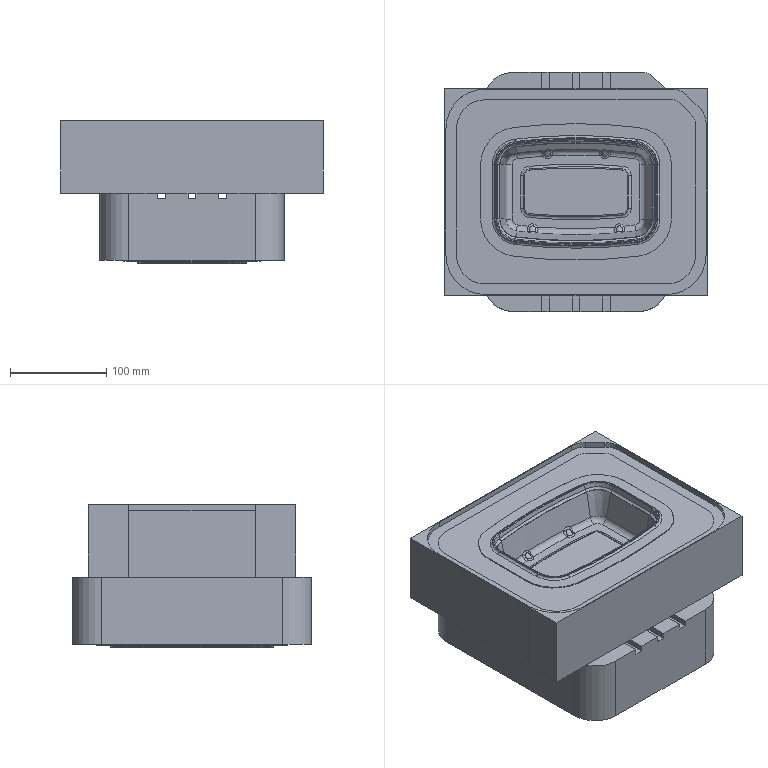NC program | NX | posted with a generic post | part box 272.387 x 248.388 x 148.5 mm
Lines 1 to 1186 of 133013:
N10 G17 G21 G94 G90
(CAVITY_MILL_1 , TOOL : D16R0.8)
N12 T00 M6
N14 G53
N16 G17 G0 G90 X-26.555 Y98.736 S7000 M3 M8
N18 G43 Z133. H0
N20 Z76.5
N22 G94 G1 X0. Z75.108 F4500.
N24 X100.052
N26 G2 X109.203 Y94.945 R12.942
N28 G1 X123.345 Y80.803
N30 G2 X127.136 Y71.651 R12.942
N32 G1 Y-65.794
N34 G2 X94.194 Y-98.736 R32.942
N36 G1 X-94.194
N38 G2 X-127.136 Y-65.794 R32.942
N40 G1 Y65.794
N42 G2 X-94.194 Y98.736 R32.942
N44 G1 X0.
N46 Y88.656
N48 X100.052
N50 G2 X102.076 Y87.817 R2.862
N52 G1 X116.218 Y73.675
N54 G2 X117.056 Y71.651 R2.862
N56 G1 Y-65.794
N58 G2 X94.194 Y-88.656 R22.862
N60 G1 X-94.194
N62 G2 X-117.056 Y-65.794 R22.862
N64 G1 Y65.794
N66 G2 X-94.194 Y88.656 R22.862
N68 G1 X0.
N70 Y78.576
N72 X97.062
N74 X106.976 Y68.662
N76 Y-65.794
N78 G2 X94.194 Y-78.576 R12.782
N80 G1 X-94.194
N82 G2 X-106.976 Y-65.794 R12.782
N84 G1 Y65.794
N86 G2 X-94.194 Y78.576 R12.782
N88 G1 X0.
N90 Y68.496
N92 X92.887
N94 X96.896 Y64.486
N96 Y-65.794
N98 G2 X94.194 Y-68.496 R2.702
N100 G1 X-94.194
N102 G2 X-96.896 Y-65.794 R2.702
N104 G1 Y65.794
N106 G2 X-94.194 Y68.496 R2.702
N108 G1 X0.
N110 Y58.416
N112 X86.816
N114 Y-58.416
N116 X-86.816
N118 Y58.416
N120 X0.
N122 Y48.336
N124 X76.736
N126 Y-48.336
N128 X-76.736
N130 Y48.336
N132 X0.
N134 Y38.256
N136 X66.656
N138 Y-38.256
N140 X-66.656
N142 Y38.256
N144 X0.
N146 Y28.176
N148 X56.576
N150 Y-28.176
N152 X-56.576
N154 Y28.176
N156 X0.
N158 Y18.096
N160 X46.496
N162 Y-18.096
N164 X-46.496
N166 Y18.096
N168 X0.
N170 Y8.016
N172 X36.416
N174 Y-8.016
N176 X-36.416
N178 Y8.016
N180 X0.
N182 Y0.816
N184 X29.216
N186 Y-0.816
N188 X-29.216
N190 Y0.816
N192 X0.
N194 G3 X3.2 Y4.016 R3.2
N196 G1 Z76.108
N198 G0 Z78.5
N200 X-26.555 Y98.644
N202 Z76.108
N204 G1 X0. Z74.717
N206 X100.052
N208 G2 X109.138 Y94.88 R12.85
N210 G1 X123.251 Y80.767
N212 X123.296 Y80.722
N214 G2 X127.044 Y71.651 R12.85
N216 G1 Y-65.794
N218 G2 X94.194 Y-98.644 R32.85
N220 G1 X-94.194
N222 G2 X-127.044 Y-65.794 R32.85
N224 G1 Y65.794
N226 G2 X-94.194 Y98.644 R32.85
N228 G1 X0.
N230 Y88.564
N232 X100.052
N234 G2 X102.01 Y87.752 R2.77
N236 G1 X116.123 Y73.64
N238 G2 X116.964 Y71.651 R2.77
N240 G1 Y-65.794
N242 G2 X94.194 Y-88.564 R22.77
N244 G1 X-94.194
N246 G2 X-116.964 Y-65.794 R22.77
N248 G1 Y65.794
N250 G2 X-94.194 Y88.564 R22.77
N252 G1 X0.
N254 Y78.484
N256 X97.024
N258 X106.884 Y68.624
N260 Y-65.794
N262 G2 X94.194 Y-78.484 R12.69
N264 G1 X-94.194
N266 G2 X-106.884 Y-65.794 R12.69
N268 G1 Y65.794
N270 G2 X-94.194 Y78.484 R12.69
N272 G1 X0.
N274 Y68.404
N276 X92.849
N278 X96.804 Y64.448
N280 Y-65.794
N282 G2 X94.194 Y-68.404 R2.61
N284 G1 X-94.194
N286 G2 X-96.804 Y-65.794 R2.61
N288 G1 Y65.794
N290 G2 X-94.194 Y68.404 R2.61
N292 G1 X0.
N294 Y58.324
N296 X86.724
N298 Y-58.324
N300 X-86.724
N302 Y58.324
N304 X0.
N306 Y48.244
N308 X76.644
N310 Y-48.244
N312 X-76.644
N314 Y48.244
N316 X0.
N318 Y38.164
N320 X66.564
N322 Y-38.164
N324 X-66.564
N326 Y38.164
N328 X0.
N330 Y28.084
N332 X56.484
N334 Y-28.084
N336 X-56.484
N338 Y28.084
N340 X0.
N342 Y18.004
N344 X46.404
N346 Y-18.004
N348 X-46.404
N350 Y18.004
N352 X0.
N354 Y7.924
N356 X36.324
N358 Y-7.924
N360 X-36.324
N362 Y7.924
N364 X0.
N366 Y0.724
N368 X29.124
N370 Y-0.724
N372 X-29.124
N374 Y0.724
N376 X0.
N378 G3 X3.2 Y3.924 R3.2
N380 G1 Z75.717
N382 G0 Z78.108
N384 X-26.555 Y98.644
N386 Z75.717
N388 G1 X0. Z74.325
N390 X100.052
N392 G2 X109.138 Y94.88 R12.85
N394 G1 X123.28 Y80.738
N396 G2 X127.044 Y71.651 R12.85
N398 G1 Y-65.794
N400 G2 X94.194 Y-98.644 R32.85
N402 G1 X-94.194
N404 G2 X-127.044 Y-65.794 R32.85
N406 G1 Y65.794
N408 G2 X-94.194 Y98.644 R32.85
N410 G1 X0.
N412 Y88.564
N414 X100.052
N416 G2 X102.01 Y87.752 R2.77
N418 G1 X116.152 Y73.61
N420 G2 X116.964 Y71.651 R2.77
N422 G1 Y-65.794
N424 G2 X94.194 Y-88.564 R22.77
N426 G1 X-94.194
N428 G2 X-116.964 Y-65.794 R22.77
N430 G1 Y65.794
N432 G2 X-94.194 Y88.564 R22.77
N434 G1 X0.
N436 Y78.484
N438 X97.024
N440 X106.884 Y68.623
N442 Y-65.794
N444 G2 X94.194 Y-78.484 R12.69
N446 G1 X-94.194
N448 G2 X-106.884 Y-65.794 R12.69
N450 G1 Y65.794
N452 G2 X-94.194 Y78.484 R12.69
N454 G1 X0.
N456 Y68.404
N458 X92.848
N460 X96.804 Y64.448
N462 Y-65.794
N464 G2 X94.194 Y-68.404 R2.61
N466 G1 X-94.194
N468 G2 X-96.804 Y-65.794 R2.61
N470 G1 Y65.794
N472 G2 X-94.194 Y68.404 R2.61
N474 G1 X0.
N476 Y58.324
N478 X86.724
N480 Y-58.324
N482 X-86.724
N484 Y58.324
N486 X0.
N488 Y48.244
N490 X76.644
N492 Y-48.244
N494 X-76.644
N496 Y48.244
N498 X0.
N500 Y38.164
N502 X66.564
N504 Y-38.164
N506 X-66.564
N508 Y38.164
N510 X0.
N512 Y28.084
N514 X56.484
N516 Y-28.084
N518 X-56.484
N520 Y28.084
N522 X0.
N524 Y18.004
N526 X46.404
N528 Y-18.004
N530 X-46.404
N532 Y18.004
N534 X0.
N536 Y7.924
N538 X36.324
N540 Y-7.924
N542 X-36.324
N544 Y7.924
N546 X0.
N548 Y0.724
N550 X29.124
N552 Y-0.724
N554 X-29.124
N556 Y0.724
N558 X0.
N560 G3 X3.2 Y3.924 R3.2
N562 G1 Z75.325
N564 G0 Z77.717
N566 X-26.555 Y98.644
N568 Z75.325
N570 G1 X0. Z73.933
N572 X100.052
N574 G2 X109.138 Y94.88 R12.85
N576 G1 X123.28 Y80.738
N578 G2 X127.044 Y71.651 R12.85
N580 G1 Y-65.794
N582 G2 X94.194 Y-98.644 R32.85
N584 G1 X-94.194
N586 G2 X-127.044 Y-65.794 R32.85
N588 G1 Y65.794
N590 G2 X-94.194 Y98.644 R32.85
N592 G1 X0.
N594 Y88.564
N596 X100.052
N598 G2 X102.01 Y87.752 R2.77
N600 G1 X116.152 Y73.61
N602 G2 X116.964 Y71.651 R2.77
N604 G1 Y-65.794
N606 G2 X94.194 Y-88.564 R22.77
N608 G1 X-94.194
N610 G2 X-116.964 Y-65.794 R22.77
N612 G1 Y65.794
N614 G2 X-94.194 Y88.564 R22.77
N616 G1 X0.
N618 Y78.484
N620 X97.024
N622 X106.884 Y68.623
N624 Y-65.794
N626 G2 X94.194 Y-78.484 R12.69
N628 G1 X-94.194
N630 G2 X-106.884 Y-65.794 R12.69
N632 G1 Y65.794
N634 G2 X-94.194 Y78.484 R12.69
N636 G1 X0.
N638 Y68.404
N640 X92.848
N642 X96.804 Y64.448
N644 Y-65.794
N646 G2 X94.194 Y-68.404 R2.61
N648 G1 X-94.194
N650 G2 X-96.804 Y-65.794 R2.61
N652 G1 Y65.794
N654 G2 X-94.194 Y68.404 R2.61
N656 G1 X0.
N658 Y58.324
N660 X86.724
N662 Y-58.324
N664 X-86.724
N666 Y58.324
N668 X0.
N670 Y48.244
N672 X76.644
N674 Y-48.244
N676 X-76.644
N678 Y48.244
N680 X0.
N682 Y38.164
N684 X66.564
N686 Y-38.164
N688 X-66.564
N690 Y38.164
N692 X0.
N694 Y28.084
N696 X56.484
N698 Y-28.084
N700 X-56.484
N702 Y28.084
N704 X0.
N706 Y18.004
N708 X46.404
N710 Y-18.004
N712 X-46.404
N714 Y18.004
N716 X0.
N718 Y7.924
N720 X36.324
N722 Y-7.924
N724 X-36.324
N726 Y7.924
N728 X0.
N730 Y0.724
N732 X29.124
N734 Y-0.724
N736 X-29.124
N738 Y0.724
N740 X0.
N742 G3 X3.2 Y3.924 R3.2
N744 G1 Z74.933
N746 G0 Z77.325
N748 X-26.555 Y98.644
N750 Z74.933
N752 G1 X0. Z73.542
N754 X100.052
N756 G2 X109.138 Y94.88 R12.85
N758 G1 X123.28 Y80.738
N760 G2 X127.044 Y71.651 R12.85
N762 G1 Y-65.794
N764 G2 X94.194 Y-98.644 R32.85
N766 G1 X-94.194
N768 G2 X-127.044 Y-65.794 R32.85
N770 G1 Y65.794
N772 G2 X-94.194 Y98.644 R32.85
N774 G1 X0.
N776 Y88.564
N778 X100.052
N780 G2 X102.01 Y87.752 R2.77
N782 G1 X116.152 Y73.61
N784 G2 X116.964 Y71.651 R2.77
N786 G1 Y-65.794
N788 G2 X94.194 Y-88.564 R22.77
N790 G1 X-94.194
N792 G2 X-116.964 Y-65.794 R22.77
N794 G1 Y65.794
N796 G2 X-94.194 Y88.564 R22.77
N798 G1 X0.
N800 Y78.484
N802 X97.024
N804 X106.884 Y68.623
N806 Y-65.794
N808 G2 X94.194 Y-78.484 R12.69
N810 G1 X-94.194
N812 G2 X-106.884 Y-65.794 R12.69
N814 G1 Y65.794
N816 G2 X-94.194 Y78.484 R12.69
N818 G1 X0.
N820 Y68.404
N822 X92.848
N824 X96.804 Y64.448
N826 Y-65.794
N828 G2 X94.194 Y-68.404 R2.61
N830 G1 X-94.194
N832 G2 X-96.804 Y-65.794 R2.61
N834 G1 Y65.794
N836 G2 X-94.194 Y68.404 R2.61
N838 G1 X0.
N840 Y58.324
N842 X86.724
N844 Y-58.324
N846 X-86.724
N848 Y58.324
N850 X0.
N852 Y48.244
N854 X76.644
N856 Y-48.244
N858 X-76.644
N860 Y48.244
N862 X0.
N864 Y38.164
N866 X66.564
N868 Y-38.164
N870 X-66.564
N872 Y38.164
N874 X0.
N876 Y28.084
N878 X56.484
N880 Y-28.084
N882 X-56.484
N884 Y28.084
N886 X0.
N888 Y18.004
N890 X46.404
N892 Y-18.004
N894 X-46.404
N896 Y18.004
N898 X0.
N900 Y7.924
N902 X36.324
N904 Y-7.924
N906 X-36.324
N908 Y7.924
N910 X0.
N912 Y0.724
N914 X29.124
N916 Y-0.724
N918 X-29.124
N920 Y0.724
N922 X0.
N924 G3 X3.2 Y3.924 R3.2
N926 G1 Z74.542
N928 G0 Z76.933
N930 X-26.555 Y98.644
N932 Z74.542
N934 G1 X0. Z73.15
N936 X100.052
N938 G2 X109.138 Y94.88 R12.85
N940 G1 X123.28 Y80.738
N942 G2 X127.044 Y71.651 R12.85
N944 G1 Y-65.794
N946 G2 X94.194 Y-98.644 R32.85
N948 G1 X-94.194
N950 G2 X-127.044 Y-65.794 R32.85
N952 G1 Y65.794
N954 G2 X-94.194 Y98.644 R32.85
N956 G1 X0.
N958 Y88.564
N960 X100.052
N962 G2 X102.01 Y87.752 R2.77
N964 G1 X116.152 Y73.61
N966 G2 X116.964 Y71.651 R2.77
N968 G1 Y-65.794
N970 G2 X94.194 Y-88.564 R22.77
N972 G1 X-94.194
N974 G2 X-116.964 Y-65.794 R22.77
N976 G1 Y65.794
N978 G2 X-94.194 Y88.564 R22.77
N980 G1 X0.
N982 Y78.484
N984 X97.024
N986 X106.884 Y68.623
N988 Y-65.794
N990 G2 X94.194 Y-78.484 R12.69
N992 G1 X-94.194
N994 G2 X-106.884 Y-65.794 R12.69
N996 G1 Y65.794
N998 G2 X-94.194 Y78.484 R12.69
N1000 G1 X0.
N1002 Y68.404
N1004 X92.848
N1006 X96.804 Y64.448
N1008 Y-65.794
N1010 G2 X94.194 Y-68.404 R2.61
N1012 G1 X-94.194
N1014 G2 X-96.804 Y-65.794 R2.61
N1016 G1 Y65.794
N1018 G2 X-94.194 Y68.404 R2.61
N1020 G1 X0.
N1022 Y58.324
N1024 X86.724
N1026 Y-58.324
N1028 X-86.724
N1030 Y58.324
N1032 X0.
N1034 Y48.244
N1036 X76.644
N1038 Y-48.244
N1040 X-76.644
N1042 Y48.244
N1044 X0.
N1046 Y38.164
N1048 X66.564
N1050 Y-38.164
N1052 X-66.564
N1054 Y38.164
N1056 X0.
N1058 Y28.084
N1060 X56.484
N1062 Y-28.084
N1064 X-56.484
N1066 Y28.084
N1068 X0.
N1070 Y18.004
N1072 X46.404
N1074 Y-18.004
N1076 X-46.404
N1078 Y18.004
N1080 X0.
N1082 Y7.924
N1084 X36.324
N1086 Y-7.924
N1088 X-36.324
N1090 Y7.924
N1092 X0.
N1094 Y0.724
N1096 X29.124
N1098 Y-0.724
N1100 X-29.124
N1102 Y0.724
N1104 X0.
N1106 G3 X3.2 Y3.924 R3.2
N1108 G1 Z74.15
N1110 G0 Z76.542
N1112 X-26.373 Y98.644
N1114 Z74.15
N1116 G1 X0. Z72.768
N1118 X100.052
N1120 G2 X109.138 Y94.88 R12.85
N1122 G1 X123.28 Y80.738
N1124 G2 X127.044 Y71.651 R12.85
N1126 G1 Y-65.794
N1128 G2 X94.194 Y-98.644 R32.85
N1130 G1 X-94.194
N1132 G2 X-127.044 Y-65.794 R32.85
N1134 G1 Y65.794
N1136 G2 X-94.194 Y98.644 R32.85
N1138 G1 X0.
N1140 Y88.564
N1142 X100.052
N1144 G2 X102.01 Y87.752 R2.77
N1146 G1 X116.152 Y73.61
N1148 G2 X116.964 Y71.651 R2.77
N1150 G1 Y-65.794
N1152 G2 X94.194 Y-88.564 R22.77
N1154 G1 X-94.194
N1156 G2 X-116.964 Y-65.794 R22.77
N1158 G1 Y65.794
N1160 G2 X-94.194 Y88.564 R22.77
N1162 G1 X0.
N1164 Y78.484
N1166 X97.024
N1168 X106.884 Y68.623
N1170 Y-65.794
N1172 G2 X94.194 Y-78.484 R12.69
N1174 G1 X-94.194
N1176 G2 X-106.884 Y-65.794 R12.69
N1178 G1 Y65.794
N1180 G2 X-94.194 Y78.484 R12.69
N1182 G1 X0.
N1184 Y68.404
N1186 X92.848
N1188 X96.804 Y64.448
N1190 Y49.668
N1192 X86.724
N1194 G3 X76.172 Y58.324 R34.054
N1196 G1 X69.25 Y61.133
N1198 X76.172 Y58.324
N1200 X86.724
N1202 Y49.668
N1204 X96.804
N1206 Y-65.794
N1208 G2 X94.194 Y-68.404 R2.61
N1210 G1 X76.392
N1212 Y-58.324
N1214 G3 X86.724 Y-49.919 R33.509
N1216 G1 Y-58.324
N1218 X76.392
N1220 X69.418 Y-61.124
N1222 X76.392 Y-58.324
N1224 Y-68.404
N1226 X-94.194
N1228 G2 X-96.804 Y-65.794 R2.61
N1230 G1 Y-49.668
N1232 X-86.724
N1234 G3 X-76.172 Y-58.324 R34.054
N1236 G1 X-69.25 Y-61.133
N1238 X-76.172 Y-58.324
N1240 X-86.724
N1242 Y-49.668
N1244 X-96.804
N1246 Y65.794
N1248 G2 X-94.194 Y68.404 R2.61
N1250 G1 X-76.172
N1252 Y58.324
N1254 G3 X-86.724 Y49.668 R34.054
N1256 G1 X-85.159 Y48.397
N1258 G2 X-64.169 Y60.003 R32.038
N1260 X64.169 Y60.003 R526.731
N1262 X92.327 Y28.201 R32.038
N1264 G1 Y-28.645
N1266 G2 X66.064 Y-59.701 R31.493
N1268 G1 X64.545 Y-59.957
N1270 G2 X-64.193 Y-60. R526.731
N1272 X-92.327 Y-28.201 R32.038
N1274 G1 Y28.201
N1276 G2 X-85.159 Y48.397 R32.038
N1278 G1 X-86.724 Y49.668
N1280 Y58.324
N1282 X-76.172
N1284 X-69.25 Y61.133
N1286 X-76.172 Y58.324
N1288 Y68.404
N1290 X0.
N1292 G3 X3.2 Y71.604 R3.2
N1294 G1 Z73.768
N1296 G0 Z76.15
N1298 X-26.373 Y98.644
N1300 Z73.768
N1302 G1 X0. Z72.386
N1304 X100.052
N1306 G2 X109.138 Y94.88 R12.85
N1308 G1 X123.28 Y80.738
N1310 G2 X127.044 Y71.651 R12.85
N1312 G1 Y-65.794
N1314 G2 X94.194 Y-98.644 R32.85
N1316 G1 X-94.194
N1318 G2 X-127.044 Y-65.794 R32.85
N1320 G1 Y65.794
N1322 G2 X-94.194 Y98.644 R32.85
N1324 G1 X0.
N1326 Y88.564
N1328 X100.052
N1330 G2 X102.01 Y87.752 R2.77
N1332 G1 X116.152 Y73.61
N1334 G2 X116.964 Y71.651 R2.77
N1336 G1 Y-65.794
N1338 G2 X94.194 Y-88.564 R22.77
N1340 G1 X-94.194
N1342 G2 X-116.964 Y-65.794 R22.77
N1344 G1 Y65.794
N1346 G2 X-94.194 Y88.564 R22.77
N1348 G1 X0.
N1350 Y78.484
N1352 X97.024
N1354 X106.884 Y68.623
N1356 Y-65.794
N1358 G2 X94.194 Y-78.484 R12.69
N1360 G1 X-94.194
N1362 G2 X-106.884 Y-65.794 R12.69
N1364 G1 Y65.794
N1366 G2 X-94.194 Y78.484 R12.69
N1368 G1 X0.
N1370 Y68.404
N1372 X92.848
N1374 X96.804 Y64.448
N1376 Y50.136
N1378 X86.724
N1380 G3 X76.799 Y58.324 R34.351
N1382 G1 X70.058 Y61.17
N1384 X76.799 Y58.324
N1386 X86.724
N1388 Y50.136
N1390 X96.804
N1392 Y-65.794
N1394 G2 X94.194 Y-68.404 R2.61
N1396 G1 X77.038
N1398 Y-58.324
N1400 G3 X86.724 Y-50.398 R33.78
N1402 G1 Y-58.324
N1404 X77.038
N1406 X70.259 Y-61.162
N1408 X77.038 Y-58.324
N1410 Y-68.404
N1412 X-94.194
N1414 G2 X-96.804 Y-65.794 R2.61
N1416 G1 Y-50.136
N1418 X-86.724
N1420 G3 X-76.799 Y-58.324 R34.351
N1422 G1 X-70.058 Y-61.17
N1424 X-76.799 Y-58.324
N1426 X-86.724
N1428 Y-50.136
N1430 X-96.804
N1432 Y65.794
N1434 G2 X-94.194 Y68.404 R2.61
N1436 G1 X-76.799
N1438 Y58.324
N1440 G3 X-86.724 Y50.136 R34.351
N1442 G1 X-85.172 Y48.849
N1444 G2 X-64.229 Y60.295 R32.335
N1446 X64.229 Y60.295 R527.028
N1448 X92.623 Y28.201 R32.335
N1450 G1 Y-28.519
N1452 G2 X86.607 Y-47.271 R32.261
N1454 X68.014 Y-59.618 R31.764
N1456 X64.582 Y-60.251 R32.117
N1458 X-64.229 Y-60.295 R527.028
N1460 X-92.623 Y-28.201 R32.335
N1462 G1 Y28.201
N1464 G2 X-85.172 Y48.849 R32.335
N1466 G1 X-86.724 Y50.136
N1468 Y58.324
N1470 X-76.799
N1472 X-70.058 Y61.17
N1474 X-76.799 Y58.324
N1476 Y68.404
N1478 X0.
N1480 G3 X3.2 Y71.604 R3.2
N1482 G1 Z73.386
N1484 G0 Z75.768
N1486 X-26.373 Y98.644
N1488 Z73.386
N1490 G1 X0. Z72.004
N1492 X100.052
N1494 G2 X109.138 Y94.88 R12.85
N1496 G1 X123.28 Y80.738
N1498 G2 X127.044 Y71.651 R12.85
N1500 G1 Y-65.794
N1502 G2 X94.194 Y-98.644 R32.85
N1504 G1 X-94.194
N1506 G2 X-127.044 Y-65.794 R32.85
N1508 G1 Y65.794
N1510 G2 X-94.194 Y98.644 R32.85
N1512 G1 X0.
N1514 Y88.564
N1516 X100.052
N1518 G2 X102.01 Y87.752 R2.77
N1520 G1 X116.152 Y73.61
N1522 G2 X116.964 Y71.651 R2.77
N1524 G1 Y-65.794
N1526 G2 X94.194 Y-88.564 R22.77
N1528 G1 X-94.194
N1530 G2 X-116.964 Y-65.794 R22.77
N1532 G1 Y65.794
N1534 G2 X-94.194 Y88.564 R22.77
N1536 G1 X0.
N1538 Y78.484
N1540 X97.024
N1542 X106.884 Y68.623
N1544 Y-65.794
N1546 G2 X94.194 Y-78.484 R12.69
N1548 G1 X-94.194
N1550 G2 X-106.884 Y-65.794 R12.69
N1552 G1 Y65.794
N1554 G2 X-94.194 Y78.484 R12.69
N1556 G1 X0.
N1558 Y68.404
N1560 X92.848
N1562 X96.804 Y64.448
N1564 Y50.355
N1566 X86.724
N1568 G3 X77.089 Y58.324 R34.491
N1570 G1 X70.423 Y61.187
N1572 X77.089 Y58.324
N1574 X86.724
N1576 Y50.355
N1578 X96.804
N1580 Y-65.794
N1582 G2 X94.194 Y-68.404 R2.61
N1584 G1 X77.341
N1586 Y-58.324
N1588 G3 X86.724 Y-50.629 R33.991
N1590 G1 Y-58.324
N1592 X77.341
N1594 X70.647 Y-61.181
N1596 X77.341 Y-58.324
N1598 Y-68.404
N1600 X-94.194
N1602 G2 X-96.804 Y-65.794 R2.61
N1604 G1 Y-50.355
N1606 X-86.724
N1608 G3 X-77.089 Y-58.324 R34.491
N1610 G1 X-70.423 Y-61.187
N1612 X-77.089 Y-58.324
N1614 X-86.724
N1616 Y-50.355
N1618 X-96.804
N1620 Y65.794
N1622 G2 X-94.194 Y68.404 R2.61
N1624 G1 X-77.089
N1626 Y58.324
N1628 G3 X-86.724 Y50.355 R34.491
N1630 G1 X-85.179 Y49.06
N1632 G2 X-64.246 Y60.434 R32.475
N1634 X64.246 Y60.434 R527.168
N1636 X92.764 Y28.201 R32.475
N1638 G1 Y-28.519
N1640 G2 X85.629 Y-48.793 R32.324
N1642 X67.035 Y-59.981 R31.975
N1644 G1 X65.078 Y-60.325
N1646 X64.599 Y-60.39
N1648 G2 X-64.246 Y-60.434 R527.168
N1650 X-92.764 Y-28.201 R32.475
N1652 G1 Y28.201
N1654 G2 X-85.179 Y49.06 R32.475
N1656 G1 X-86.724 Y50.355
N1658 Y58.324
N1660 X-77.089
N1662 X-70.423 Y61.187
N1664 X-77.089 Y58.324
N1666 Y68.404
N1668 X0.
N1670 G3 X3.2 Y71.604 R3.2
N1672 G1 Z73.004
N1674 G0 Z75.386
N1676 X-26.373 Y98.644
N1678 Z73.004
N1680 G1 X0. Z71.621
N1682 X100.052
N1684 G2 X109.138 Y94.88 R12.85
N1686 G1 X123.28 Y80.738
N1688 G2 X127.044 Y71.651 R12.85
N1690 G1 Y-65.794
N1692 G2 X94.194 Y-98.644 R32.85
N1694 G1 X-94.194
N1696 G2 X-127.044 Y-65.794 R32.85
N1698 G1 Y65.794
N1700 G2 X-94.194 Y98.644 R32.85
N1702 G1 X0.
N1704 Y88.564
N1706 X100.052
N1708 G2 X102.01 Y87.752 R2.77
N1710 G1 X116.152 Y73.61
N1712 G2 X116.964 Y71.651 R2.77
N1714 G1 Y-65.794
N1716 G2 X94.194 Y-88.564 R22.77
N1718 G1 X-94.194
N1720 G2 X-116.964 Y-65.794 R22.77
N1722 G1 Y65.794
N1724 G2 X-94.194 Y88.564 R22.77
N1726 G1 X0.
N1728 Y78.484
N1730 X97.024
N1732 X106.884 Y68.623
N1734 Y-65.794
N1736 G2 X94.194 Y-78.484 R12.69
N1738 G1 X-94.194
N1740 G2 X-106.884 Y-65.794 R12.69
N1742 G1 Y65.794
N1744 G2 X-94.194 Y78.484 R12.69
N1746 G1 X0.
N1748 Y68.404
N1750 X92.848
N1752 X96.804 Y64.448
N1754 Y50.553
N1756 X86.724
N1758 G3 X77.349 Y58.324 R34.619
N1760 G1 X86.724
N1762 Y50.553
N1764 X96.804
N1766 Y-65.794
N1768 G2 X94.194 Y-68.404 R2.61
N1770 G1 X77.646
N1772 Y-58.324
N1774 G3 X86.724 Y-50.852 R34.118
N1776 G1 Y-58.324
N1778 X77.646
N1780 Y-68.404
N1782 X-94.194
N1784 G2 X-96.804 Y-65.794 R2.61
N1786 G1 Y-50.553
N1788 X-86.724
N1790 G3 X-77.349 Y-58.324 R34.619
N1792 G1 X-86.724
N1794 Y-50.553
N1796 X-96.804
N1798 Y65.794
N1800 G2 X-94.194 Y68.404 R2.61
N1802 G1 X-77.349
N1804 Y58.324
N1806 G3 X-86.724 Y50.553 R34.619
N1808 G1 X-85.184 Y49.251
N1810 G2 X-64.262 Y60.56 R32.603
N1812 X64.262 Y60.56 R527.296
N1814 X92.891 Y28.201 R32.603
N1816 G1 Y-28.472
N1818 X92.914 Y-28.511
N1820 X92.873 Y-29.731
N1822 G2 X86.607 Y-47.768 R32.229
N1824 X64.57 Y-60.523 R32.102
N1826 X-64.262 Y-60.56 R527.296
N1828 X-92.891 Y-28.201 R32.603
N1830 G1 Y28.201
N1832 G2 X-85.184 Y49.251 R32.603
N1834 G1 X-86.724 Y50.553
N1836 Y58.324
N1838 X-77.349
N1840 Y68.404
N1842 X0.
N1844 G3 X3.2 Y71.604 R3.2
N1846 G1 Z72.621
N1848 G0 Z75.004
N1850 X-26.373 Y98.644
N1852 Z72.621
N1854 G1 X0. Z71.239
N1856 X100.052
N1858 G2 X109.138 Y94.88 R12.85
N1860 G1 X123.28 Y80.738
N1862 G2 X127.044 Y71.651 R12.85
N1864 G1 Y-65.794
N1866 G2 X94.194 Y-98.644 R32.85
N1868 G1 X-94.194
N1870 G2 X-127.044 Y-65.794 R32.85
N1872 G1 Y65.794
N1874 G2 X-94.194 Y98.644 R32.85
N1876 G1 X0.
N1878 Y88.564
N1880 X100.052
N1882 G2 X102.01 Y87.752 R2.77
N1884 G1 X116.152 Y73.61
N1886 G2 X116.964 Y71.651 R2.77
N1888 G1 Y-65.794
N1890 G2 X94.194 Y-88.564 R22.77
N1892 G1 X-94.194
N1894 G2 X-116.964 Y-65.794 R22.77
N1896 G1 Y65.794
N1898 G2 X-94.194 Y88.564 R22.77
N1900 G1 X0.
N1902 Y78.484
N1904 X97.024
N1906 X106.884 Y68.623
N1908 Y-65.794
N1910 G2 X94.194 Y-78.484 R12.69
N1912 G1 X-94.194
N1914 G2 X-106.884 Y-65.794 R12.69
N1916 G1 Y65.794
N1918 G2 X-94.194 Y78.484 R12.69
N1920 G1 X0.
N1922 Y68.404
N1924 X92.848
N1926 X96.804 Y64.448
N1928 Y51.009
N1930 X86.724
N1932 G3 X77.942 Y58.324 R34.915
N1934 G1 X86.724
N1936 Y51.009
N1938 X96.804
N1940 Y-65.794
N1942 G2 X94.194 Y-68.404 R2.61
N1944 G1 X78.255
N1946 Y-58.324
N1948 G3 X86.724 Y-51.309 R34.329
N1950 G1 Y-58.324
N1952 X78.255
N1954 Y-68.404
N1956 X-94.194
N1958 G2 X-96.804 Y-65.794 R2.61
N1960 G1 Y-51.009
N1962 X-86.724
N1964 G3 X-77.942 Y-58.324 R34.915
N1966 G1 X-86.724
N1968 Y-51.009
N1970 X-96.804
N1972 Y65.794
N1974 G2 X-94.194 Y68.404 R2.61
N1976 G1 X-77.942
N1978 Y58.324
N1980 G3 X-86.724 Y51.009 R34.915
N1982 G1 X-85.197 Y49.692
N1984 G2 X-64.298 Y60.854 R32.899
N1986 X64.298 Y60.854 R527.592
N1988 X93.187 Y28.201 R32.899
N1990 G1 Y-28.501
N1992 G2 X64.592 Y-60.818 R32.313
N1994 X-64.298 Y-60.854 R527.592
N1996 X-93.187 Y-28.201 R32.899
N1998 G1 Y28.201
N2000 G2 X-85.197 Y49.692 R32.899
N2002 G1 X-86.724 Y51.009
N2004 Y58.324
N2006 X-77.942
N2008 Y68.404
N2010 X0.
N2012 G3 X3.2 Y71.604 R3.2
N2014 G1 Z72.239
N2016 G0 Z74.621
N2018 X-26.373 Y98.644
N2020 Z72.239
N2022 G1 X0. Z70.857
N2024 X100.052
N2026 G2 X109.138 Y94.88 R12.85
N2028 G1 X123.28 Y80.738
N2030 G2 X127.044 Y71.651 R12.85
N2032 G1 Y-65.794
N2034 G2 X94.194 Y-98.644 R32.85
N2036 G1 X-94.194
N2038 G2 X-127.044 Y-65.794 R32.85
N2040 G1 Y65.794
N2042 G2 X-94.194 Y98.644 R32.85
N2044 G1 X0.
N2046 Y88.564
N2048 X100.052
N2050 G2 X102.01 Y87.752 R2.77
N2052 G1 X116.152 Y73.61
N2054 G2 X116.964 Y71.651 R2.77
N2056 G1 Y-65.794
N2058 G2 X94.194 Y-88.564 R22.77
N2060 G1 X-94.194
N2062 G2 X-116.964 Y-65.794 R22.77
N2064 G1 Y65.794
N2066 G2 X-94.194 Y88.564 R22.77
N2068 G1 X0.
N2070 Y78.484
N2072 X97.024
N2074 X106.884 Y68.623
N2076 Y-65.794
N2078 G2 X94.194 Y-78.484 R12.69
N2080 G1 X-94.194
N2082 G2 X-106.884 Y-65.794 R12.69
N2084 G1 Y65.794
N2086 G2 X-94.194 Y78.484 R12.69
N2088 G1 X0.
N2090 Y68.404
N2092 X92.848
N2094 X96.804 Y64.448
N2096 Y52.263
N2098 X86.724
N2100 G3 X79.535 Y58.324 R35.747
N2102 G1 X86.724
N2104 Y52.263
N2106 X96.804
N2108 Y-65.794
N2110 G2 X94.194 Y-68.404 R2.61
N2112 G1 X80.035
N2114 Y-58.324
N2116 G3 X86.724 Y-52.732 R34.798
N2118 G1 Y-58.324
N2120 X80.035
N2122 Y-68.404
N2124 X-94.194
N2126 G2 X-96.804 Y-65.794 R2.61
N2128 G1 Y-52.263
N2130 X-86.724
N2132 G3 X-79.535 Y-58.324 R35.747
N2134 G1 X-86.724
N2136 Y-52.263
N2138 X-96.804
N2140 Y65.794
N2142 G2 X-94.194 Y68.404 R2.61
N2144 G1 X-79.535
N2146 Y58.324
N2148 G3 X-86.724 Y52.263 R35.747
N2150 G1 X-85.233 Y50.906
N2152 G2 X-64.399 Y61.68 R33.731
N2154 X64.399 Y61.68 R528.424
N2156 X94.019 Y28.201 R33.731
N2158 G1 Y-29.039
N2160 G2 X65.287 Y-61.57 R32.782
N2162 X-64.399 Y-61.68 R528.424
N2164 X-94.019 Y-28.201 R33.731
N2166 G1 Y28.201
N2168 G2 X-85.233 Y50.906 R33.731
N2170 G1 X-86.724 Y52.263
N2172 Y58.324
N2174 X-79.535
N2176 Y68.404
N2178 X0.
N2180 G3 X3.2 Y71.604 R3.2
N2182 G1 Z71.857
N2184 G0 Z74.239
N2186 X-25.442 Y98.644
N2188 Z71.857
N2190 G1 X0. Z70.524
N2192 X100.052
N2194 G2 X109.138 Y94.88 R12.85
N2196 G1 X123.28 Y80.738
N2198 G2 X127.044 Y71.651 R12.85
N2200 G1 Y-65.794
N2202 G2 X94.194 Y-98.644 R32.85
N2204 G1 X-94.194
N2206 G2 X-127.044 Y-65.794 R32.85
N2208 G1 Y65.794
N2210 G2 X-94.194 Y98.644 R32.85
N2212 G1 X0.
N2214 Y88.564
N2216 X100.052
N2218 G2 X102.01 Y87.752 R2.77
N2220 G1 X116.152 Y73.61
N2222 G2 X116.964 Y71.651 R2.77
N2224 G1 Y42.85
N2226 X106.884
N2228 G3 X66.241 Y76.681 R48.844
N2230 X49.39 Y78.484 R543.537
N2232 G1 X97.024
N2234 X106.884 Y68.623
N2236 Y42.85
N2238 X108.531 Y35.841
N2240 G2 X109.132 Y28.201 R48.844
N2242 G1 Y-28.201
N2244 G2 X108.531 Y-35.841 R48.844
N2246 X109.764 Y-36.251 R7.2
N2248 G1 Y36.251
N2250 G2 X108.531 Y35.841 R7.2
N2252 G1 X106.884 Y42.85
N2254 X116.964
N2256 Y-65.794
N2258 G2 X94.194 Y-88.564 R22.77
N2260 G1 X49.39
N2262 Y-78.484
N2264 G3 X66.183 Y-76.688 R543.537
N2266 X106.884 Y-42.85 R48.844
N2268 G1 Y-65.794
N2270 G2 X100.994 Y-76.508 R12.69
N2272 G1 X97.136 Y-70.429
N2274 G3 X98.502 Y-69.197 R56.044
N2276 G2 X97.136 Y-70.429 R5.49
N2278 G1 X100.994 Y-76.508
N2280 G2 X94.194 Y-78.484 R12.69
N2282 G1 X49.39
N2284 Y-88.564
N2286 X-94.194
N2288 G2 X-116.964 Y-65.794 R22.77
N2290 G1 Y-42.85
N2292 X-106.884
N2294 G3 X-66.273 Y-76.677 R48.844
N2296 X-49.39 Y-78.484 R543.537
N2298 G1 X-42.791 Y-81.364
N2300 X42.791
N2302 G2 X42.216 Y-79.09 R7.2
N2304 X-42.216 Y-79.09 R543.537
N2306 X-42.791 Y-81.364 R7.2
N2308 G1 X-49.39 Y-78.484
N2310 X-94.194
N2312 G2 X-104.152 Y-73.66 R12.69
N2314 G1 X-98.502 Y-69.197
N2316 G3 X-97.136 Y-70.429 R56.044
N2318 G2 X-98.502 Y-69.197 R5.49
N2320 G1 X-104.152 Y-73.66
N2322 G2 X-106.884 Y-65.794 R12.69
N2324 G1 Y-42.85
N2326 X-108.531 Y-35.841
N2328 G2 X-109.132 Y-28.201 R48.844
N2330 G1 Y28.201
N2332 G2 X-108.531 Y35.841 R48.844
N2334 X-109.764 Y36.251 R7.2
N2336 G1 Y-36.251
N2338 G2 X-108.531 Y-35.841 R7.2
N2340 G1 X-106.884 Y-42.85
N2342 X-116.964
N2344 Y65.794
N2346 G2 X-94.194 Y88.564 R22.77
N2348 G1 X-49.39
N2350 Y78.484
N2352 G3 X-66.183 Y76.688 R543.537
N2354 X-106.884 Y42.85 R48.844
N2356 G1 X-104.961 Y42.246
N2358 G2 X-66.026 Y74.676 R46.828
N2360 G1 X-65.938 Y74.687
N2362 G2 X65.995 Y74.68 R541.521
N2364 X107.116 Y28.201 R46.828
N2366 G1 Y-28.201
N2368 G2 X66.026 Y-74.676 R46.828
N2370 G1 X65.938 Y-74.687